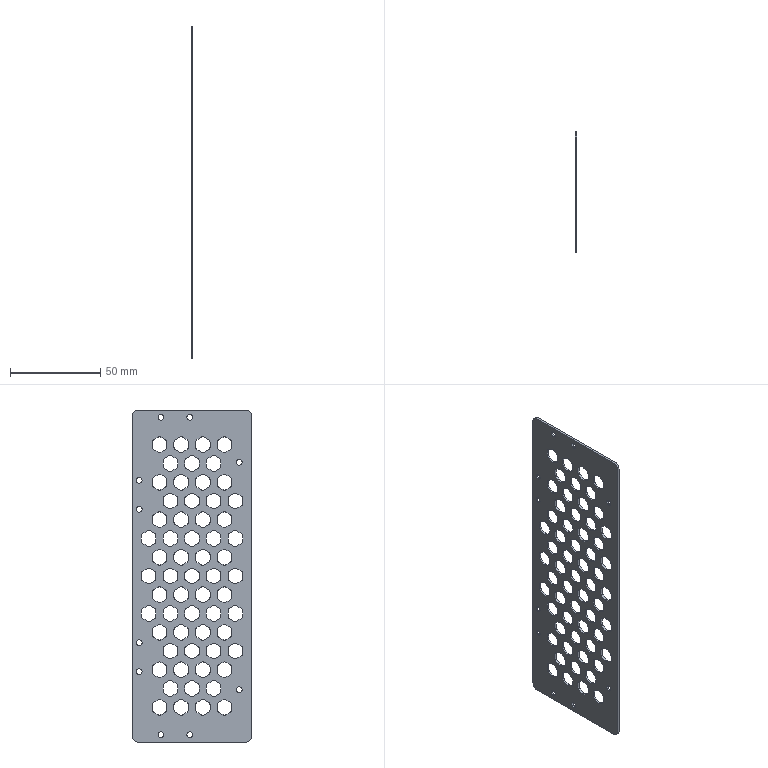Part | SolidWorks | features Fillet 2, ICE 2, APattern 1, Extrusion 1 | 1 solid | 823 faces | box 1 x 66.5 x 184 mm | volume 8811 mm3 | cylinder 451 | plane 372 | commonest cylinder face diameters 3 x427 3.2 x20 6 x4